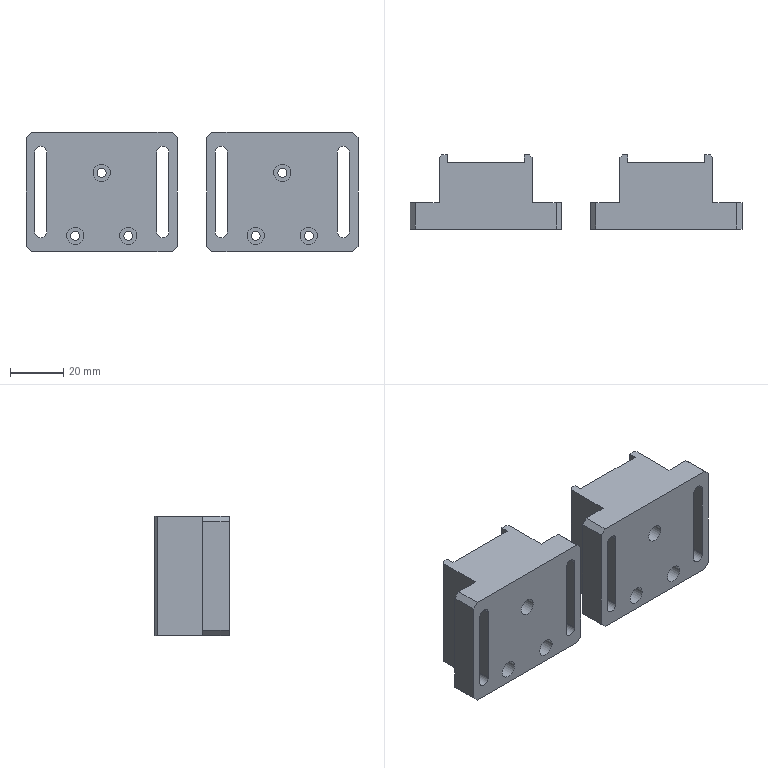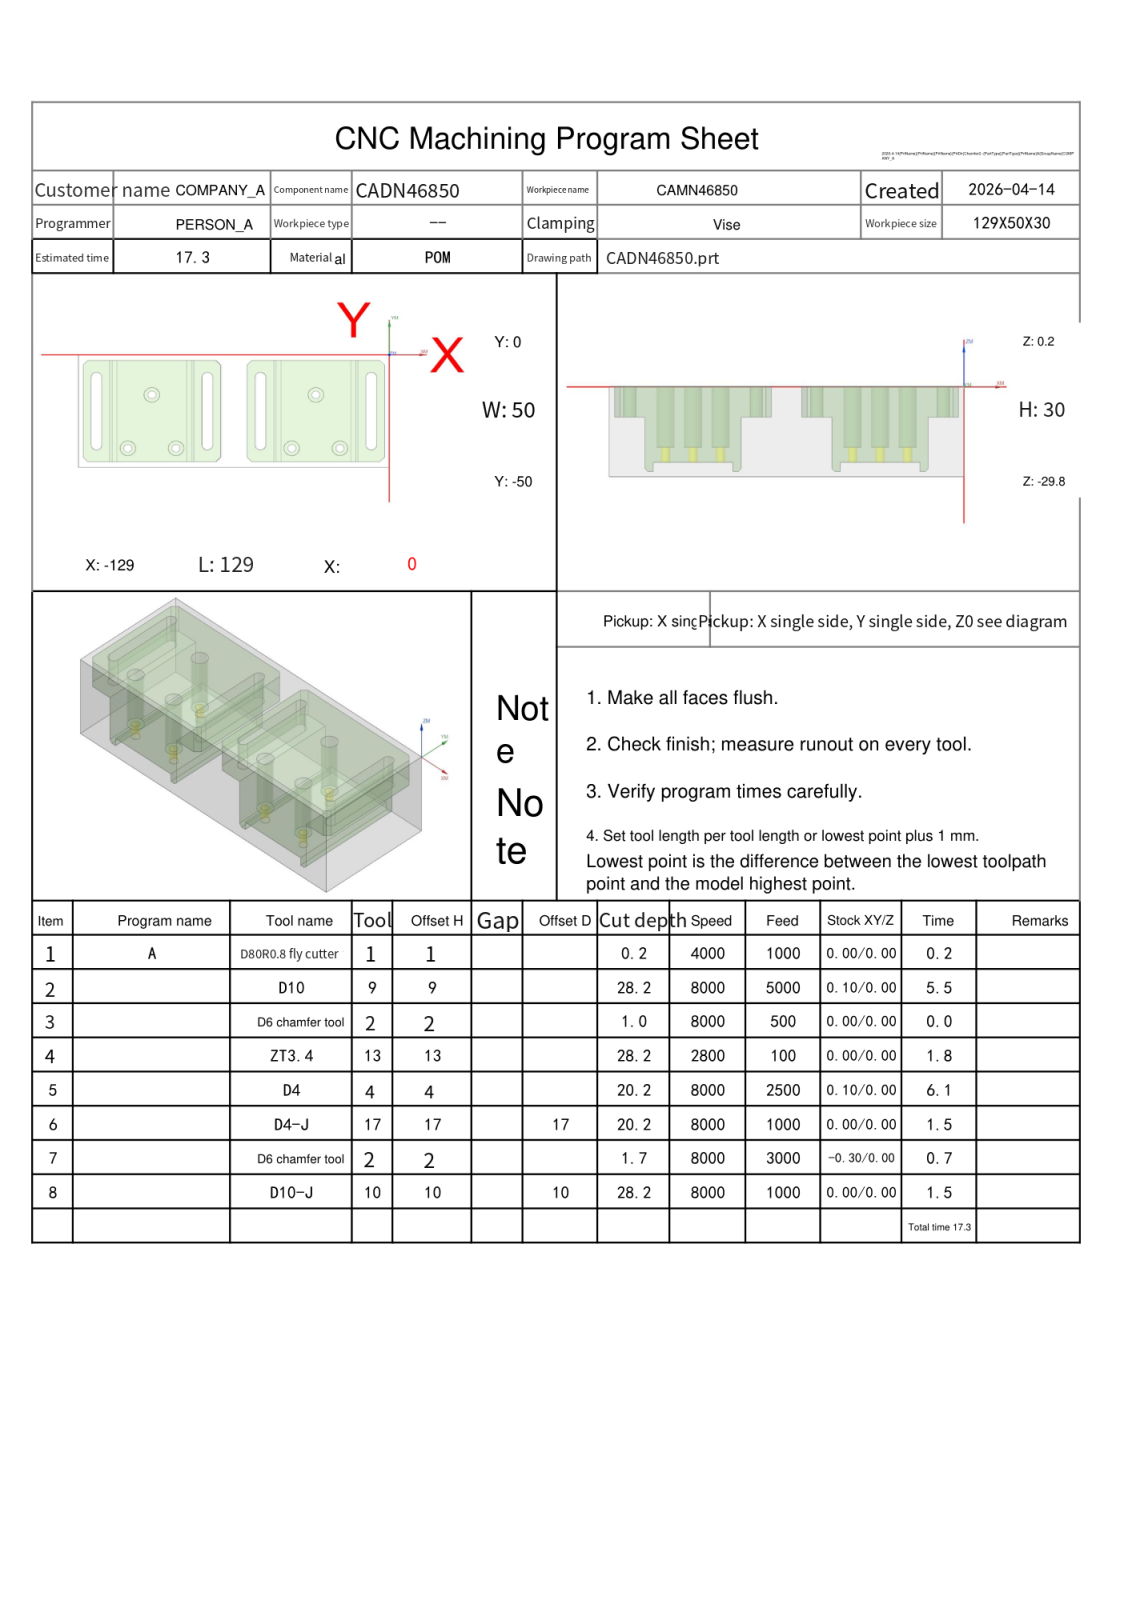NC program | NX | posted by the shop | part box 125 x 28 x 45 mm
Lines 34 to 804 of 4607:
N2 T09 M06
(D10  D=10. R=0. H=09 ce=0.10 di=0.00)
G00 G90 G54 X-30.5 Y-52.6 M03 S8000
G43 H09 Z20.
M08
Z.5
G01 X-57. Z.444 F5000.
G02 X-60.606 Y-51.106 Z.435 I0.0 J5.1
G01 X-62.606 Y-49.106 Z.429
G02 X-64.1 Y-45.5 Z.421 I3.606 J3.606
G01 Y-4.5 Z.334
G02 X-62.606 Y-.894 Z.325 I5.1 J0.0
G01 X-60.606 Y1.106 Z.319
G02 X-57. Y2.6 Z.311 I3.606 J-3.606
G01 X-4. Z.198
G02 X-.394 Y1.106 Z.19 I0.0 J-5.1
G01 X1.606 Y-.894 Z.184
G02 X3.1 Y-4.5 Z.175 I-3.606 J-3.606
G01 Y-45.5 Z.088
G02 X1.606 Y-49.106 Z.079 I-5.1 J0.0
G01 X-.394 Y-51.106 Z.073
G02 X-4. Y-52.6 Z.065 I-3.606 J3.606
G01 X-57. Z-.048
G02 X-60.606 Y-51.106 Z-.056 I0.0 J5.1
G01 X-62.606 Y-49.106 Z-.062
G02 X-64.1 Y-45.5 Z-.071 I3.606 J3.606
G01 Y-4.5 Z-.158
G02 X-62.606 Y-.894 Z-.166 I5.1 J0.0
G01 X-60.606 Y1.106 Z-.172
G02 X-57. Y2.6 Z-.181 I3.606 J-3.606
G01 X-4. Z-.293
G02 X-.394 Y1.106 Z-.302 I0.0 J-5.1
G01 X1.606 Y-.894 Z-.308
G02 X3.1 Y-4.5 Z-.316 I-3.606 J-3.606
G01 Y-45.5 Z-.403
G02 X1.606 Y-49.106 Z-.412 I-5.1 J0.0
G01 X-.394 Y-51.106 Z-.418
G02 X-4. Y-52.6 Z-.426 I-3.606 J3.606
G01 X-57. Z-.539
G02 X-60.606 Y-51.106 Z-.548 I0.0 J5.1
G01 X-62.606 Y-49.106 Z-.554
G02 X-64.1 Y-45.5 Z-.562 I3.606 J3.606
G01 Y-4.5 Z-.649
G02 X-62.606 Y-.894 Z-.658 I5.1 J0.0
G01 X-60.606 Y1.106 Z-.664
G02 X-57. Y2.6 Z-.672 I3.606 J-3.606
G01 X-4. Z-.785
G02 X-.394 Y1.106 Z-.793 I0.0 J-5.1
G01 X1.606 Y-.894 Z-.799
G02 X3.1 Y-4.5 Z-.808 I-3.606 J-3.606
G01 Y-45.5 Z-.895
G02 X1.606 Y-49.106 Z-.903 I-5.1 J0.0
G01 X-.394 Y-51.106 Z-.909
G02 X-4. Y-52.6 Z-.918 I-3.606 J3.606
G01 X-57. Z-1.03
G02 X-60.606 Y-51.106 Z-1.039 I0.0 J5.1
G01 X-62.606 Y-49.106 Z-1.045
G02 X-64.1 Y-45.5 Z-1.053 I3.606 J3.606
G01 Y-4.5 Z-1.141
G02 X-62.606 Y-.894 Z-1.149 I5.1 J0.0
G01 X-60.606 Y1.106 Z-1.155
G02 X-57. Y2.6 Z-1.164 I3.606 J-3.606
G01 X-4. Z-1.276
G02 X-.394 Y1.106 Z-1.285 I0.0 J-5.1
G01 X1.606 Y-.894 Z-1.291
G02 X3.1 Y-4.5 Z-1.299 I-3.606 J-3.606
G01 Y-45.5 Z-1.386
G02 X1.606 Y-49.106 Z-1.395 I-5.1 J0.0
G01 X-.394 Y-51.106 Z-1.401
G02 X-4. Y-52.6 Z-1.409 I-3.606 J3.606
G01 X-57. Z-1.522
G02 X-60.606 Y-51.106 Z-1.53 I0.0 J5.1
G01 X-62.606 Y-49.106 Z-1.536
G02 X-64.1 Y-45.5 Z-1.545 I3.606 J3.606
G01 Y-4.5 Z-1.632
G02 X-62.606 Y-.894 Z-1.64 I5.1 J0.0
G01 X-60.606 Y1.106 Z-1.646
G02 X-57. Y2.6 Z-1.655 I3.606 J-3.606
G01 X-4. Z-1.767
G02 X-.394 Y1.106 Z-1.776 I0.0 J-5.1
G01 X1.606 Y-.894 Z-1.782
G02 X3.1 Y-4.5 Z-1.791 I-3.606 J-3.606
G01 Y-45.5 Z-1.878
G02 X1.606 Y-49.106 Z-1.886 I-5.1 J0.0
G01 X-.394 Y-51.106 Z-1.892
G02 X-4. Y-52.6 Z-1.901 I-3.606 J3.606
G01 X-57. Z-2.013
G02 X-60.606 Y-51.106 Z-2.022 I0.0 J5.1
G01 X-62.606 Y-49.106 Z-2.028
G02 X-64.1 Y-45.5 Z-2.036 I3.606 J3.606
G01 Y-4.5 Z-2.123
G02 X-62.606 Y-.894 Z-2.132 I5.1 J0.0
G01 X-60.606 Y1.106 Z-2.138
G02 X-57. Y2.6 Z-2.146 I3.606 J-3.606
G01 X-4. Z-2.259
G02 X-.394 Y1.106 Z-2.267 I0.0 J-5.1
G01 X1.606 Y-.894 Z-2.273
G02 X3.1 Y-4.5 Z-2.282 I-3.606 J-3.606
G01 Y-45.5 Z-2.369
G02 X1.606 Y-49.106 Z-2.377 I-5.1 J0.0
G01 X-.394 Y-51.106 Z-2.383
G02 X-4. Y-52.6 Z-2.392 I-3.606 J3.606
G01 X-57. Z-2.505
G02 X-60.606 Y-51.106 Z-2.513 I0.0 J5.1
G01 X-62.606 Y-49.106 Z-2.519
G02 X-64.1 Y-45.5 Z-2.528 I3.606 J3.606
G01 Y-4.5 Z-2.615
G02 X-62.606 Y-.894 Z-2.623 I5.1 J0.0
G01 X-60.606 Y1.106 Z-2.629
G02 X-57. Y2.6 Z-2.638 I3.606 J-3.606
G01 X-4. Z-2.75
G02 X-.394 Y1.106 Z-2.759 I0.0 J-5.1
G01 X1.606 Y-.894 Z-2.765
G02 X3.1 Y-4.5 Z-2.773 I-3.606 J-3.606
G01 Y-45.5 Z-2.86
G02 X1.606 Y-49.106 Z-2.869 I-5.1 J0.0
G01 X-.394 Y-51.106 Z-2.875
G02 X-4. Y-52.6 Z-2.883 I-3.606 J3.606
G01 X-57. Z-2.996
G02 X-60.606 Y-51.106 Z-3.004 I0.0 J5.1
G01 X-62.606 Y-49.106 Z-3.01
G02 X-64.1 Y-45.5 Z-3.019 I3.606 J3.606
G01 Y-4.5 Z-3.106
G02 X-62.606 Y-.894 Z-3.115 I5.1 J0.0
G01 X-60.606 Y1.106 Z-3.121
G02 X-57. Y2.6 Z-3.129 I3.606 J-3.606
G01 X-4. Z-3.242
G02 X-.394 Y1.106 Z-3.25 I0.0 J-5.1
G01 X1.606 Y-.894 Z-3.256
G02 X3.1 Y-4.5 Z-3.265 I-3.606 J-3.606
G01 Y-45.5 Z-3.352
G02 X1.606 Y-49.106 Z-3.36 I-5.1 J0.0
G01 X-.394 Y-51.106 Z-3.366
G02 X-4. Y-52.6 Z-3.375 I-3.606 J3.606
G01 X-57. Z-3.487
G02 X-60.606 Y-51.106 Z-3.496 I0.0 J5.1
G01 X-62.606 Y-49.106 Z-3.502
G02 X-64.1 Y-45.5 Z-3.51 I3.606 J3.606
G01 Y-4.5 Z-3.597
G02 X-62.606 Y-.894 Z-3.606 I5.1 J0.0
G01 X-60.606 Y1.106 Z-3.612
G02 X-57. Y2.6 Z-3.62 I3.606 J-3.606
G01 X-4. Z-3.733
G02 X-.394 Y1.106 Z-3.742 I0.0 J-5.1
G01 X1.606 Y-.894 Z-3.748
G02 X3.1 Y-4.5 Z-3.756 I-3.606 J-3.606
G01 Y-45.5 Z-3.843
G02 X1.606 Y-49.106 Z-3.852 I-5.1 J0.0
G01 X-.394 Y-51.106 Z-3.858
G02 X-4. Y-52.6 Z-3.866 I-3.606 J3.606
G01 X-57. Z-3.979
G02 X-60.606 Y-51.106 Z-3.987 I0.0 J5.1
G01 X-62.606 Y-49.106 Z-3.993
G02 X-64.1 Y-45.5 Z-4.002 I3.606 J3.606
G01 Y-4.5 Z-4.089
G02 X-62.606 Y-.894 Z-4.097 I5.1 J0.0
G01 X-60.606 Y1.106 Z-4.103
G02 X-57. Y2.6 Z-4.112 I3.606 J-3.606
G01 X-4. Z-4.224
G02 X-.394 Y1.106 Z-4.233 I0.0 J-5.1
G01 X1.606 Y-.894 Z-4.239
G02 X3.1 Y-4.5 Z-4.247 I-3.606 J-3.606
G01 Y-45.5 Z-4.334
G02 X1.606 Y-49.106 Z-4.343 I-5.1 J0.0
G01 X-.394 Y-51.106 Z-4.349
G02 X-4. Y-52.6 Z-4.358 I-3.606 J3.606
G01 X-57. Z-4.47
G02 X-60.606 Y-51.106 Z-4.479 I0.0 J5.1
G01 X-62.606 Y-49.106 Z-4.485
G02 X-64.1 Y-45.5 Z-4.493 I3.606 J3.606
G01 Y-4.5 Z-4.58
G02 X-62.606 Y-.894 Z-4.589 I5.1 J0.0
G01 X-60.606 Y1.106 Z-4.595
G02 X-57. Y2.6 Z-4.603 I3.606 J-3.606
G01 X-4. Z-4.716
G02 X-.394 Y1.106 Z-4.724 I0.0 J-5.1
G01 X1.606 Y-.894 Z-4.73
G02 X3.1 Y-4.5 Z-4.739 I-3.606 J-3.606
G01 Y-45.5 Z-4.826
G02 X1.606 Y-49.106 Z-4.834 I-5.1 J0.0
G01 X-.394 Y-51.106 Z-4.84
G02 X-4. Y-52.6 Z-4.849 I-3.606 J3.606
G01 X-57. Z-4.961
G02 X-60.606 Y-51.106 Z-4.97 I0.0 J5.1
G01 X-62.606 Y-49.106 Z-4.976
G02 X-64.1 Y-45.5 Z-4.984 I3.606 J3.606
G01 Y-4.5 Z-5.072
G02 X-62.606 Y-.894 Z-5.08 I5.1 J0.0
G01 X-60.606 Y1.106 Z-5.086
G02 X-57. Y2.6 Z-5.095 I3.606 J-3.606
G01 X-4. Z-5.207
G02 X-.394 Y1.106 Z-5.216 I0.0 J-5.1
G01 X1.606 Y-.894 Z-5.222
G02 X3.1 Y-4.5 Z-5.23 I-3.606 J-3.606
G01 Y-45.5 Z-5.317
G02 X1.606 Y-49.106 Z-5.326 I-5.1 J0.0
G01 X-.394 Y-51.106 Z-5.332
G02 X-4. Y-52.6 Z-5.34 I-3.606 J3.606
G01 X-57. Z-5.453
G02 X-60.606 Y-51.106 Z-5.461 I0.0 J5.1
G01 X-62.606 Y-49.106 Z-5.467
G02 X-64.1 Y-45.5 Z-5.476 I3.606 J3.606
G01 Y-4.5 Z-5.563
G02 X-62.606 Y-.894 Z-5.571 I5.1 J0.0
G01 X-60.606 Y1.106 Z-5.577
G02 X-57. Y2.6 Z-5.586 I3.606 J-3.606
G01 X-4. Z-5.699
G02 X-.394 Y1.106 Z-5.707 I0.0 J-5.1
G01 X1.606 Y-.894 Z-5.713
G02 X3.1 Y-4.5 Z-5.722 I-3.606 J-3.606
G01 Y-45.5 Z-5.809
G02 X1.606 Y-49.106 Z-5.817 I-5.1 J0.0
G01 X-.394 Y-51.106 Z-5.823
G02 X-4. Y-52.6 Z-5.832 I-3.606 J3.606
G01 X-57. Z-5.944
G02 X-60.606 Y-51.106 Z-5.953 I0.0 J5.1
G01 X-62.606 Y-49.106 Z-5.959
G02 X-64.1 Y-45.5 Z-5.967 I3.606 J3.606
G01 Y-4.5 Z-6.054
G02 X-62.606 Y-.894 Z-6.063 I5.1 J0.0
G01 X-60.606 Y1.106 Z-6.069
G02 X-57. Y2.6 Z-6.077 I3.606 J-3.606
G01 X-4. Z-6.19
G02 X-.394 Y1.106 Z-6.198 I0.0 J-5.1
G01 X1.606 Y-.894 Z-6.204
G02 X3.1 Y-4.5 Z-6.213 I-3.606 J-3.606
G01 Y-45.5 Z-6.3
G02 X1.606 Y-49.106 Z-6.309 I-5.1 J0.0
G01 X-.394 Y-51.106 Z-6.315
G02 X-4. Y-52.6 Z-6.323 I-3.606 J3.606
G01 X-57. Z-6.436
G02 X-60.606 Y-51.106 Z-6.444 I0.0 J5.1
G01 X-62.606 Y-49.106 Z-6.45
G02 X-64.1 Y-45.5 Z-6.459 I3.606 J3.606
G01 Y-4.5 Z-6.546
G02 X-62.606 Y-.894 Z-6.554 I5.1 J0.0
G01 X-60.606 Y1.106 Z-6.56
G02 X-57. Y2.6 Z-6.569 I3.606 J-3.606
G01 X-4. Z-6.681
G02 X-.394 Y1.106 Z-6.69 I0.0 J-5.1
G01 X1.606 Y-.894 Z-6.696
G02 X3.1 Y-4.5 Z-6.704 I-3.606 J-3.606
G01 Y-45.5 Z-6.791
G02 X1.606 Y-49.106 Z-6.8 I-5.1 J0.0
G01 X-.394 Y-51.106 Z-6.806
G02 X-4. Y-52.6 Z-6.814 I-3.606 J3.606
G01 X-57. Z-6.927
G02 X-60.606 Y-51.106 Z-6.935 I0.0 J5.1
G01 X-62.606 Y-49.106 Z-6.941
G02 X-64.1 Y-45.5 Z-6.95 I3.606 J3.606
G01 Y-4.5 Z-7.037
G02 X-62.606 Y-.894 Z-7.046 I5.1 J0.0
G01 X-60.606 Y1.106 Z-7.052
G02 X-57. Y2.6 Z-7.06 I3.606 J-3.606
G01 X-4. Z-7.173
G02 X-.394 Y1.106 Z-7.181 I0.0 J-5.1
G01 X1.606 Y-.894 Z-7.187
G02 X3.1 Y-4.5 Z-7.196 I-3.606 J-3.606
G01 Y-45.5 Z-7.283
G02 X1.606 Y-49.106 Z-7.291 I-5.1 J0.0
G01 X-.394 Y-51.106 Z-7.297
G02 X-4. Y-52.6 Z-7.306 I-3.606 J3.606
G01 X-57. Z-7.418
G02 X-60.606 Y-51.106 Z-7.427 I0.0 J5.1
G01 X-62.606 Y-49.106 Z-7.433
G02 X-64.1 Y-45.5 Z-7.441 I3.606 J3.606
G01 Y-4.5 Z-7.528
G02 X-62.606 Y-.894 Z-7.537 I5.1 J0.0
G01 X-60.606 Y1.106 Z-7.543
G02 X-57. Y2.6 Z-7.551 I3.606 J-3.606
G01 X-4. Z-7.664
G02 X-.394 Y1.106 Z-7.673 I0.0 J-5.1
G01 X1.606 Y-.894 Z-7.679
G02 X3.1 Y-4.5 Z-7.687 I-3.606 J-3.606
G01 Y-45.5 Z-7.774
G02 X1.606 Y-49.106 Z-7.783 I-5.1 J0.0
G01 X-.394 Y-51.106 Z-7.789
G02 X-4. Y-52.6 Z-7.797 I-3.606 J3.606
G01 X-57. Z-7.91
G02 X-60.606 Y-51.106 Z-7.918 I0.0 J5.1
G01 X-62.606 Y-49.106 Z-7.924
G02 X-64.1 Y-45.5 Z-7.933 I3.606 J3.606
G01 Y-4.5 Z-8.02
G02 X-62.606 Y-.894 Z-8.028 I5.1 J0.0
G01 X-60.606 Y1.106 Z-8.034
G02 X-57. Y2.6 Z-8.043 I3.606 J-3.606
G01 X-4. Z-8.155
G02 X-.394 Y1.106 Z-8.164 I0.0 J-5.1
G01 X1.606 Y-.894 Z-8.17
G02 X3.1 Y-4.5 Z-8.178 I-3.606 J-3.606
G01 Y-45.5 Z-8.266
G02 X1.606 Y-49.106 Z-8.274 I-5.1 J0.0
G01 X-.394 Y-51.106 Z-8.28
G02 X-4. Y-52.6 Z-8.289 I-3.606 J3.606
G01 X-57. Z-8.401
G02 X-60.606 Y-51.106 Z-8.41 I0.0 J5.1
G01 X-62.606 Y-49.106 Z-8.416
G02 X-64.1 Y-45.5 Z-8.424 I3.606 J3.606
G01 Y-4.5 Z-8.511
G02 X-62.606 Y-.894 Z-8.52 I5.1 J0.0
G01 X-60.606 Y1.106 Z-8.526
G02 X-57. Y2.6 Z-8.534 I3.606 J-3.606
G01 X-4. Z-8.647
G02 X-.394 Y1.106 Z-8.655 I0.0 J-5.1
G01 X1.606 Y-.894 Z-8.661
G02 X3.1 Y-4.5 Z-8.67 I-3.606 J-3.606
G01 Y-45.5 Z-8.757
G02 X1.606 Y-49.106 Z-8.765 I-5.1 J0.0
G01 X-.394 Y-51.106 Z-8.771
G02 X-4. Y-52.6 Z-8.78 I-3.606 J3.606
G01 X-57. Z-8.892
G02 X-60.606 Y-51.106 Z-8.901 I0.0 J5.1
G01 X-62.606 Y-49.106 Z-8.907
G02 X-64.1 Y-45.5 Z-8.916 I3.606 J3.606
G01 Y-4.5 Z-9.003
G02 X-62.606 Y-.894 Z-9.011 I5.1 J0.0
G01 X-60.606 Y1.106 Z-9.017
G02 X-57. Y2.6 Z-9.026 I3.606 J-3.606
G01 X-4. Z-9.138
G02 X-.394 Y1.106 Z-9.147 I0.0 J-5.1
G01 X1.606 Y-.894 Z-9.153
G02 X3.1 Y-4.5 Z-9.161 I-3.606 J-3.606
G01 Y-45.5 Z-9.248
G02 X1.606 Y-49.106 Z-9.257 I-5.1 J0.0
G01 X-.394 Y-51.106 Z-9.263
G02 X-4. Y-52.6 Z-9.271 I-3.606 J3.606
G01 X-57. Z-9.384
G02 X-60.606 Y-51.106 Z-9.392 I0.0 J5.1
G01 X-62.606 Y-49.106 Z-9.398
G02 X-64.1 Y-45.5 Z-9.407 I3.606 J3.606
G01 Y-4.5 Z-9.494
G02 X-62.606 Y-.894 Z-9.502 I5.1 J0.0
G01 X-60.606 Y1.106 Z-9.508
G02 X-57. Y2.6 Z-9.517 I3.606 J-3.606
G01 X-4. Z-9.63
G02 X-.394 Y1.106 Z-9.638 I0.0 J-5.1
G01 X1.606 Y-.894 Z-9.644
G02 X3.1 Y-4.5 Z-9.653 I-3.606 J-3.606
G01 Y-45.5 Z-9.74
G02 X1.606 Y-49.106 Z-9.748 I-5.1 J0.0
G01 X-.394 Y-51.106 Z-9.754
G02 X-4. Y-52.6 Z-9.763 I-3.606 J3.606
G01 X-57. Z-9.875
G02 X-60.606 Y-51.106 Z-9.884 I0.0 J5.1
G01 X-62.606 Y-49.106 Z-9.89
G02 X-64.1 Y-45.5 Z-9.898 I3.606 J3.606
G01 Y-4.5 Z-9.985
G02 X-62.606 Y-.894 Z-9.994 I5.1 J0.0
G01 X-60.606 Y1.106 Z-10.
G02 X-57. Y2.6 Z-10.008 I3.606 J-3.606
G01 X-4. Z-10.121
G02 X-.394 Y1.106 Z-10.129 I0.0 J-5.1
G01 X1.606 Y-.894 Z-10.135
G02 X3.1 Y-4.5 Z-10.144 I-3.606 J-3.606
G01 Y-45.5 Z-10.231
G02 X1.606 Y-49.106 Z-10.24 I-5.1 J0.0
G01 X-.394 Y-51.106 Z-10.246
G02 X-4. Y-52.6 Z-10.254 I-3.606 J3.606
G01 X-57. Z-10.367
G02 X-60.606 Y-51.106 Z-10.375 I0.0 J5.1
G01 X-62.606 Y-49.106 Z-10.381
G02 X-64.1 Y-45.5 Z-10.39 I3.606 J3.606
G01 Y-4.5 Z-10.477
G02 X-62.606 Y-.894 Z-10.485 I5.1 J0.0
G01 X-60.606 Y1.106 Z-10.491
G02 X-57. Y2.6 Z-10.5 I3.606 J-3.606
G01 X-4. Z-10.612
G02 X-.394 Y1.106 Z-10.621 I0.0 J-5.1
G01 X1.606 Y-.894 Z-10.627
G02 X3.1 Y-4.5 Z-10.635 I-3.606 J-3.606
G01 Y-45.5 Z-10.722
G02 X1.606 Y-49.106 Z-10.731 I-5.1 J0.0
G01 X-.394 Y-51.106 Z-10.737
G02 X-4. Y-52.6 Z-10.745 I-3.606 J3.606
G01 X-57. Z-10.858
G02 X-60.606 Y-51.106 Z-10.867 I0.0 J5.1
G01 X-62.606 Y-49.106 Z-10.873
G02 X-64.1 Y-45.5 Z-10.881 I3.606 J3.606
G01 Y-4.5 Z-10.968
G02 X-62.606 Y-.894 Z-10.977 I5.1 J0.0
G01 X-60.606 Y1.106 Z-10.983
G02 X-57. Y2.6 Z-10.991 I3.606 J-3.606
G01 X-4. Z-11.104
G02 X-.394 Y1.106 Z-11.112 I0.0 J-5.1
G01 X1.606 Y-.894 Z-11.118
G02 X3.1 Y-4.5 Z-11.127 I-3.606 J-3.606
G01 Y-45.5 Z-11.214
G02 X1.606 Y-49.106 Z-11.222 I-5.1 J0.0
G01 X-.394 Y-51.106 Z-11.228
G02 X-4. Y-52.6 Z-11.237 I-3.606 J3.606
G01 X-57. Z-11.349
G02 X-60.606 Y-51.106 Z-11.358 I0.0 J5.1
G01 X-62.606 Y-49.106 Z-11.364
G02 X-64.1 Y-45.5 Z-11.372 I3.606 J3.606
G01 Y-4.5 Z-11.459
G02 X-62.606 Y-.894 Z-11.468 I5.1 J0.0
G01 X-60.606 Y1.106 Z-11.474
G02 X-57. Y2.6 Z-11.483 I3.606 J-3.606
G01 X-4. Z-11.595
G02 X-.394 Y1.106 Z-11.604 I0.0 J-5.1
G01 X1.606 Y-.894 Z-11.61
G02 X3.1 Y-4.5 Z-11.618 I-3.606 J-3.606
G01 Y-45.5 Z-11.705
G02 X1.606 Y-49.106 Z-11.714 I-5.1 J0.0
G01 X-.394 Y-51.106 Z-11.72
G02 X-4. Y-52.6 Z-11.728 I-3.606 J3.606
G01 X-57. Z-11.841
G02 X-60.606 Y-51.106 Z-11.849 I0.0 J5.1
G01 X-62.606 Y-49.106 Z-11.855
G02 X-64.1 Y-45.5 Z-11.864 I3.606 J3.606
G01 Y-4.5 Z-11.951
G02 X-62.606 Y-.894 Z-11.959 I5.1 J0.0
G01 X-60.606 Y1.106 Z-11.965
G02 X-57. Y2.6 Z-11.974 I3.606 J-3.606
G01 X-4. Z-12.086
G02 X-.394 Y1.106 Z-12.095 I0.0 J-5.1
G01 X1.606 Y-.894 Z-12.101
G02 X3.1 Y-4.5 Z-12.109 I-3.606 J-3.606
G01 Y-45.5 Z-12.197
G02 X1.606 Y-49.106 Z-12.205 I-5.1 J0.0
G01 X-.394 Y-51.106 Z-12.211
G02 X-4. Y-52.6 Z-12.22 I-3.606 J3.606
G01 X-57. Z-12.332
G02 X-60.606 Y-51.106 Z-12.341 I0.0 J5.1
G01 X-62.606 Y-49.106 Z-12.347
G02 X-64.1 Y-45.5 Z-12.355 I3.606 J3.606
G01 Y-4.5 Z-12.442
G02 X-62.606 Y-.894 Z-12.451 I5.1 J0.0
G01 X-60.606 Y1.106 Z-12.457
G02 X-57. Y2.6 Z-12.465 I3.606 J-3.606
G01 X-4. Z-12.578
G02 X-.394 Y1.106 Z-12.586 I0.0 J-5.1
G01 X1.606 Y-.894 Z-12.592
G02 X3.1 Y-4.5 Z-12.601 I-3.606 J-3.606
G01 Y-45.5 Z-12.688
G02 X1.606 Y-49.106 Z-12.696 I-5.1 J0.0
G01 X-.394 Y-51.106 Z-12.702
G02 X-4. Y-52.6 Z-12.711 I-3.606 J3.606
G01 X-57. Z-12.824
G02 X-60.606 Y-51.106 Z-12.832 I0.0 J5.1
G01 X-62.606 Y-49.106 Z-12.838
G02 X-64.1 Y-45.5 Z-12.847 I3.606 J3.606
G01 Y-4.5 Z-12.934
G02 X-62.606 Y-.894 Z-12.942 I5.1 J0.0
G01 X-60.606 Y1.106 Z-12.948
G02 X-57. Y2.6 Z-12.957 I3.606 J-3.606
G01 X-4. Z-13.069
G02 X-.394 Y1.106 Z-13.078 I0.0 J-5.1
G01 X1.606 Y-.894 Z-13.084
G02 X3.1 Y-4.5 Z-13.092 I-3.606 J-3.606
G01 Y-45.5 Z-13.179
G02 X1.606 Y-49.106 Z-13.188 I-5.1 J0.0
G01 X-.394 Y-51.106 Z-13.194
G02 X-4. Y-52.6 Z-13.202 I-3.606 J3.606
G01 X-57. Z-13.315
G02 X-60.606 Y-51.106 Z-13.323 I0.0 J5.1
G01 X-62.606 Y-49.106 Z-13.329
G02 X-64.1 Y-45.5 Z-13.338 I3.606 J3.606
G01 Y-4.5 Z-13.425
G02 X-62.606 Y-.894 Z-13.434 I5.1 J0.0
G01 X-60.606 Y1.106 Z-13.44
G02 X-57. Y2.6 Z-13.448 I3.606 J-3.606
G01 X-4. Z-13.561
G02 X-.394 Y1.106 Z-13.569 I0.0 J-5.1
G01 X1.606 Y-.894 Z-13.575
G02 X3.1 Y-4.5 Z-13.584 I-3.606 J-3.606
G01 Y-45.5 Z-13.671
G02 X1.606 Y-49.106 Z-13.679 I-5.1 J0.0
G01 X-.394 Y-51.106 Z-13.685
G02 X-4. Y-52.6 Z-13.694 I-3.606 J3.606
G01 X-57. Z-13.806
G02 X-60.606 Y-51.106 Z-13.815 I0.0 J5.1
G01 X-62.606 Y-49.106 Z-13.821
G02 X-64.1 Y-45.5 Z-13.829 I3.606 J3.606
G01 Y-4.5 Z-13.916
G02 X-62.606 Y-.894 Z-13.925 I5.1 J0.0
G01 X-60.606 Y1.106 Z-13.931
G02 X-57. Y2.6 Z-13.939 I3.606 J-3.606
G01 X-4. Z-14.052
G02 X-.394 Y1.106 Z-14.06 I0.0 J-5.1
G01 X1.606 Y-.894 Z-14.066
G02 X3.1 Y-4.5 Z-14.075 I-3.606 J-3.606
G01 Y-45.5 Z-14.162
G02 X1.606 Y-49.106 Z-14.171 I-5.1 J0.0
G01 X-.394 Y-51.106 Z-14.177
G02 X-4. Y-52.6 Z-14.185 I-3.606 J3.606
G01 X-57. Z-14.298
G02 X-60.606 Y-51.106 Z-14.306 I0.0 J5.1
G01 X-62.606 Y-49.106 Z-14.312
G02 X-64.1 Y-45.5 Z-14.321 I3.606 J3.606
G01 Y-4.5 Z-14.408
G02 X-62.606 Y-.894 Z-14.416 I5.1 J0.0
G01 X-60.606 Y1.106 Z-14.422
G02 X-57. Y2.6 Z-14.431 I3.606 J-3.606
G01 X-4. Z-14.543
G02 X-.394 Y1.106 Z-14.552 I0.0 J-5.1
G01 X1.606 Y-.894 Z-14.558
G02 X3.1 Y-4.5 Z-14.566 I-3.606 J-3.606
G01 Y-45.5 Z-14.653
G02 X1.606 Y-49.106 Z-14.662 I-5.1 J0.0
G01 X-.394 Y-51.106 Z-14.668
G02 X-4. Y-52.6 Z-14.676 I-3.606 J3.606
G01 X-57. Z-14.789
G02 X-60.606 Y-51.106 Z-14.798 I0.0 J5.1
G01 X-62.606 Y-49.106 Z-14.804
G02 X-64.1 Y-45.5 Z-14.812 I3.606 J3.606
G01 Y-4.5 Z-14.899
G02 X-62.606 Y-.894 Z-14.908 I5.1 J0.0
G01 X-60.606 Y1.106 Z-14.914
G02 X-57. Y2.6 Z-14.922 I3.606 J-3.606
G01 X-4. Z-15.035
G02 X-.394 Y1.106 Z-15.043 I0.0 J-5.1
G01 X1.606 Y-.894 Z-15.049
G02 X3.1 Y-4.5 Z-15.058 I-3.606 J-3.606
G01 Y-45.5 Z-15.145
G02 X1.606 Y-49.106 Z-15.153 I-5.1 J0.0
G01 X-.394 Y-51.106 Z-15.159
G02 X-4. Y-52.6 Z-15.168 I-3.606 J3.606
G01 X-57. Z-15.28
G02 X-60.606 Y-51.106 Z-15.289 I0.0 J5.1
G01 X-62.606 Y-49.106 Z-15.295
G02 X-64.1 Y-45.5 Z-15.303 I3.606 J3.606
G01 Y-4.5 Z-15.391
G02 X-62.606 Y-.894 Z-15.399 I5.1 J0.0
G01 X-60.606 Y1.106 Z-15.405
G02 X-57. Y2.6 Z-15.414 I3.606 J-3.606
G01 X-4. Z-15.526
G02 X-.394 Y1.106 Z-15.535 I0.0 J-5.1
G01 X1.606 Y-.894 Z-15.541
G02 X3.1 Y-4.5 Z-15.549 I-3.606 J-3.606
G01 Y-45.5 Z-15.636
G02 X1.606 Y-49.106 Z-15.645 I-5.1 J0.0
G01 X-.394 Y-51.106 Z-15.651
G02 X-4. Y-52.6 Z-15.659 I-3.606 J3.606
G01 X-57. Z-15.772
G02 X-60.606 Y-51.106 Z-15.78 I0.0 J5.1
G01 X-62.606 Y-49.106 Z-15.786
G02 X-64.1 Y-45.5 Z-15.795 I3.606 J3.606
G01 Y-4.5 Z-15.882
G02 X-62.606 Y-.894 Z-15.89 I5.1 J0.0
G01 X-60.606 Y1.106 Z-15.896
G02 X-57. Y2.6 Z-15.905 I3.606 J-3.606
G01 X-4. Z-16.017
G02 X-.394 Y1.106 Z-16.026 I0.0 J-5.1
G01 X1.606 Y-.894 Z-16.032
G02 X3.1 Y-4.5 Z-16.041 I-3.606 J-3.606
G01 Y-45.5 Z-16.128
G02 X1.606 Y-49.106 Z-16.136 I-5.1 J0.0
G01 X-.394 Y-51.106 Z-16.142
G02 X-4. Y-52.6 Z-16.151 I-3.606 J3.606
G01 X-57. Z-16.263
G02 X-60.606 Y-51.106 Z-16.272 I0.0 J5.1
G01 X-62.606 Y-49.106 Z-16.278
G02 X-64.1 Y-45.5 Z-16.286 I3.606 J3.606
G01 Y-4.5 Z-16.373
G02 X-62.606 Y-.894 Z-16.382 I5.1 J0.0
G01 X-60.606 Y1.106 Z-16.388
G02 X-57. Y2.6 Z-16.396 I3.606 J-3.606
G01 X-4. Z-16.509
G02 X-.394 Y1.106 Z-16.517 I0.0 J-5.1
G01 X1.606 Y-.894 Z-16.523
G02 X3.1 Y-4.5 Z-16.532 I-3.606 J-3.606
G01 Y-45.5 Z-16.619
G02 X1.606 Y-49.106 Z-16.627 I-5.1 J0.0
G01 X-.394 Y-51.106 Z-16.633
G02 X-4. Y-52.6 Z-16.642 I-3.606 J3.606
G01 X-57. Z-16.755
G02 X-60.606 Y-51.106 Z-16.763 I0.0 J5.1
G01 X-62.606 Y-49.106 Z-16.769
G02 X-64.1 Y-45.5 Z-16.778 I3.606 J3.606
G01 Y-4.5 Z-16.865
G02 X-62.606 Y-.894 Z-16.873 I5.1 J0.0
G01 X-60.606 Y1.106 Z-16.879
G02 X-57. Y2.6 Z-16.888 I3.606 J-3.606
G01 X-4. Z-17.
G02 X-.394 Y1.106 Z-17.009 I0.0 J-5.1
G01 X1.606 Y-.894 Z-17.015
G02 X3.1 Y-4.5 Z-17.023 I-3.606 J-3.606
G01 Y-45.5 Z-17.11
G02 X1.606 Y-49.106 Z-17.119 I-5.1 J0.0
G01 X-.394 Y-51.106 Z-17.125
G02 X-4. Y-52.6 Z-17.133 I-3.606 J3.606
G01 X-57. Z-17.246
G02 X-60.606 Y-51.106 Z-17.254 I0.0 J5.1
G01 X-62.606 Y-49.106 Z-17.26
G02 X-64.1 Y-45.5 Z-17.269 I3.606 J3.606
G01 Y-4.5 Z-17.356
G02 X-62.606 Y-.894 Z-17.365 I5.1 J0.0
G01 X-60.606 Y1.106 Z-17.371
G02 X-57. Y2.6 Z-17.379 I3.606 J-3.606
G01 X-4. Z-17.492
G02 X-.394 Y1.106 Z-17.5 I0.0 J-5.1
G01 X1.606 Y-.894 Z-17.506
G02 X3.1 Y-4.5 Z-17.515 I-3.606 J-3.606
G01 Y-45.5 Z-17.602
G02 X1.606 Y-49.106 Z-17.61 I-5.1 J0.0
G01 X-.394 Y-51.106 Z-17.616
G02 X-4. Y-52.6 Z-17.625 I-3.606 J3.606
G01 X-57. Z-17.737
G02 X-60.606 Y-51.106 Z-17.746 I0.0 J5.1
G01 X-62.606 Y-49.106 Z-17.752
G02 X-64.1 Y-45.5 Z-17.76 I3.606 J3.606
G01 Y-4.5 Z-17.847
G02 X-62.606 Y-.894 Z-17.856 I5.1 J0.0
G01 X-60.606 Y1.106 Z-17.862
G02 X-57. Y2.6 Z-17.87 I3.606 J-3.606
G01 X-4. Z-17.983
G02 X-.394 Y1.106 Z-17.992 I0.0 J-5.1
G01 X1.606 Y-.894 Z-17.998
G02 X3.1 Y-4.5 Z-18.006 I-3.606 J-3.606
G01 Y-45.5 Z-18.093
G02 X1.606 Y-49.106 Z-18.102 I-5.1 J0.0
G01 X-.394 Y-51.106 Z-18.108
G02 X-4. Y-52.6 Z-18.116 I-3.606 J3.606
G01 X-57. Z-18.229
G02 X-60.606 Y-51.106 Z-18.237 I0.0 J5.1
G01 X-62.606 Y-49.106 Z-18.243
G02 X-64.1 Y-45.5 Z-18.252 I3.606 J3.606
G01 Y-4.5 Z-18.339
G02 X-62.606 Y-.894 Z-18.347 I5.1 J0.0
G01 X-60.606 Y1.106 Z-18.353
G02 X-57. Y2.6 Z-18.362 I3.606 J-3.606
G01 X-4. Z-18.474
G02 X-.394 Y1.106 Z-18.483 I0.0 J-5.1
G01 X1.606 Y-.894 Z-18.489
G02 X3.1 Y-4.5 Z-18.497 I-3.606 J-3.606
G01 Y-45.5 Z-18.584
G02 X1.606 Y-49.106 Z-18.593 I-5.1 J0.0
G01 X-.394 Y-51.106 Z-18.599
G02 X-4. Y-52.6 Z-18.608 I-3.606 J3.606
G01 X-57. Z-18.72
G02 X-60.606 Y-51.106 Z-18.729 I0.0 J5.1
G01 X-62.606 Y-49.106 Z-18.735
G02 X-64.1 Y-45.5 Z-18.743 I3.606 J3.606
G01 Y-4.5 Z-18.83
G02 X-62.606 Y-.894 Z-18.839 I5.1 J0.0
G01 X-60.606 Y1.106 Z-18.845
G02 X-57. Y2.6 Z-18.853 I3.606 J-3.606
G01 X-4. Z-18.966
G02 X-.394 Y1.106 Z-18.974 I0.0 J-5.1
G01 X1.606 Y-.894 Z-18.98
G02 X3.1 Y-4.5 Z-18.989 I-3.606 J-3.606
G01 Y-45.5 Z-19.076
G02 X1.606 Y-49.106 Z-19.084 I-5.1 J0.0
G01 X-.394 Y-51.106 Z-19.09
G02 X-4. Y-52.6 Z-19.099 I-3.606 J3.606
G01 X-57. Z-19.211
G02 X-60.606 Y-51.106 Z-19.22 I0.0 J5.1
G01 X-62.606 Y-49.106 Z-19.226
G02 X-64.1 Y-45.5 Z-19.234 I3.606 J3.606
G01 Y-4.5 Z-19.322
G02 X-62.606 Y-.894 Z-19.33 I5.1 J0.0
G01 X-60.606 Y1.106 Z-19.336
G02 X-57. Y2.6 Z-19.345 I3.606 J-3.606
G01 X-4. Z-19.457
G02 X-.394 Y1.106 Z-19.466 I0.0 J-5.1
G01 X1.606 Y-.894 Z-19.472
G02 X3.1 Y-4.5 Z-19.48 I-3.606 J-3.606
G01 Y-45.5 Z-19.567
G02 X1.606 Y-49.106 Z-19.576 I-5.1 J0.0
G01 X-.394 Y-51.106 Z-19.582
G02 X-4. Y-52.6 Z-19.59 I-3.606 J3.606
G01 X-57. Z-19.703
G02 X-60.606 Y-51.106 Z-19.711 I0.0 J5.1
G01 X-62.606 Y-49.106 Z-19.717
G02 X-64.1 Y-45.5 Z-19.726 I3.606 J3.606
G01 Y-4.5 Z-19.813
G02 X-62.606 Y-.894 Z-19.821 I5.1 J0.0
G01 X-60.606 Y1.106 Z-19.827
G02 X-57. Y2.6 Z-19.836 I3.606 J-3.606
G01 X-4. Z-19.949
G02 X-.394 Y1.106 Z-19.957 I0.0 J-5.1
G01 X1.606 Y-.894 Z-19.963
G02 X3.1 Y-4.5 Z-19.972 I-3.606 J-3.606
G01 Y-45.5 Z-20.059
G02 X1.606 Y-49.106 Z-20.067 I-5.1 J0.0
G01 X-.394 Y-51.106 Z-20.073
G02 X-4. Y-52.6 Z-20.082 I-3.606 J3.606
G01 X-57. Z-20.194
G02 X-60.606 Y-51.106 Z-20.203 I0.0 J5.1
G01 X-62.606 Y-49.106 Z-20.209
G02 X-64.1 Y-45.5 Z-20.217 I3.606 J3.606
G01 Y-4.5 Z-20.304
G02 X-62.606 Y-.894 Z-20.313 I5.1 J0.0
G01 X-60.606 Y1.106 Z-20.319
G02 X-57. Y2.6 Z-20.327 I3.606 J-3.606
G01 X-4. Z-20.44
G02 X-.394 Y1.106 Z-20.448 I0.0 J-5.1
G01 X1.606 Y-.894 Z-20.454
G02 X3.1 Y-4.5 Z-20.463 I-3.606 J-3.606
G01 Y-45.5 Z-20.55
G02 X1.606 Y-49.106 Z-20.559 I-5.1 J0.0
G01 X-.394 Y-51.106 Z-20.565
G02 X-4. Y-52.6 Z-20.573 I-3.606 J3.606
G01 X-57. Z-20.686
G02 X-60.606 Y-51.106 Z-20.694 I0.0 J5.1
G01 X-62.606 Y-49.106 Z-20.7
G02 X-64.1 Y-45.5 Z-20.709 I3.606 J3.606
G01 Y-4.5 Z-20.796
G02 X-62.606 Y-.894 Z-20.804 I5.1 J0.0
G01 X-60.606 Y1.106 Z-20.81
G02 X-57. Y2.6 Z-20.819 I3.606 J-3.606
G01 X-4. Z-20.931
G02 X-.394 Y1.106 Z-20.94 I0.0 J-5.1
G01 X1.606 Y-.894 Z-20.946
G02 X3.1 Y-4.5 Z-20.954 I-3.606 J-3.606
G01 Y-45.5 Z-21.041
G02 X1.606 Y-49.106 Z-21.05 I-5.1 J0.0
G01 X-.394 Y-51.106 Z-21.056
G02 X-4. Y-52.6 Z-21.064 I-3.606 J3.606
G01 X-57. Z-21.177
G02 X-60.606 Y-51.106 Z-21.185 I0.0 J5.1
G01 X-62.606 Y-49.106 Z-21.191
G02 X-64.1 Y-45.5 Z-21.2 I3.606 J3.606
G01 Y-4.5 Z-21.287
G02 X-62.606 Y-.894 Z-21.296 I5.1 J0.0
G01 X-60.606 Y1.106 Z-21.302
G02 X-57. Y2.6 Z-21.31 I3.606 J-3.606
G01 X-4. Z-21.423
G02 X-.394 Y1.106 Z-21.431 I0.0 J-5.1
G01 X1.606 Y-.894 Z-21.437
G02 X3.1 Y-4.5 Z-21.446 I-3.606 J-3.606
G01 Y-45.5 Z-21.533
G02 X1.606 Y-49.106 Z-21.541 I-5.1 J0.0
G01 X-.394 Y-51.106 Z-21.547
G02 X-4. Y-52.6 Z-21.556 I-3.606 J3.606
G01 X-57. Z-21.668
G02 X-60.606 Y-51.106 Z-21.677 I0.0 J5.1
G01 X-62.606 Y-49.106 Z-21.683
G02 X-64.1 Y-45.5 Z-21.691 I3.606 J3.606
G01 Y-4.5 Z-21.778
G02 X-62.606 Y-.894 Z-21.787 I5.1 J0.0
G01 X-60.606 Y1.106 Z-21.793
G02 X-57. Y2.6 Z-21.801 I3.606 J-3.606
G01 X-4. Z-21.914
G02 X-.394 Y1.106 Z-21.923 I0.0 J-5.1
G01 X1.606 Y-.894 Z-21.929
G02 X3.1 Y-4.5 Z-21.937 I-3.606 J-3.606
G01 Y-45.5 Z-22.024
G02 X1.606 Y-49.106 Z-22.033 I-5.1 J0.0
G01 X-.394 Y-51.106 Z-22.039
G02 X-4. Y-52.6 Z-22.047 I-3.606 J3.606
G01 X-57. Z-22.16
G02 X-60.606 Y-51.106 Z-22.168 I0.0 J5.1
G01 X-62.606 Y-49.106 Z-22.174
G02 X-64.1 Y-45.5 Z-22.183 I3.606 J3.606
G01 Y-4.5 Z-22.27
G02 X-62.606 Y-.894 Z-22.278 I5.1 J0.0
G01 X-60.606 Y1.106 Z-22.284
G02 X-57. Y2.6 Z-22.293 I3.606 J-3.606
G01 X-4. Z-22.405
G02 X-.394 Y1.106 Z-22.414 I0.0 J-5.1
G01 X1.606 Y-.894 Z-22.42
G02 X3.1 Y-4.5 Z-22.428 I-3.606 J-3.606
G01 Y-45.5 Z-22.516
G02 X1.606 Y-49.106 Z-22.524 I-5.1 J0.0
G01 X-.394 Y-51.106 Z-22.53
G02 X-4. Y-52.6 Z-22.539 I-3.606 J3.606
G01 X-57. Z-22.651
G02 X-60.606 Y-51.106 Z-22.66 I0.0 J5.1
G01 X-62.606 Y-49.106 Z-22.666
G02 X-64.1 Y-45.5 Z-22.674 I3.606 J3.606
G01 Y-4.5 Z-22.761
G02 X-62.606 Y-.894 Z-22.77 I5.1 J0.0
G01 X-60.606 Y1.106 Z-22.776
G02 X-57. Y2.6 Z-22.784 I3.606 J-3.606
G01 X-4. Z-22.897
G02 X-.394 Y1.106 Z-22.905 I0.0 J-5.1
G01 X1.606 Y-.894 Z-22.911
G02 X3.1 Y-4.5 Z-22.92 I-3.606 J-3.606
G01 Y-45.5 Z-23.007